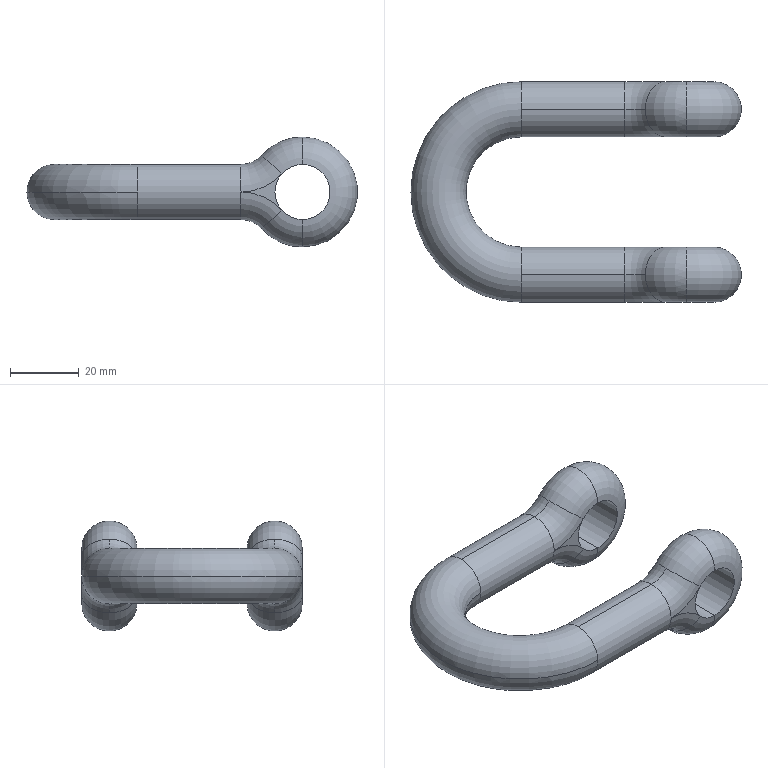Part | STEP file | TNS-16-Part-2 | 1 solid | 28 faces | box 96 x 64 x 32 mm | volume 43358 mm3 | torus 16 | cylinder 8 | plane 4 | commonest cylinder face diameters 16 x8